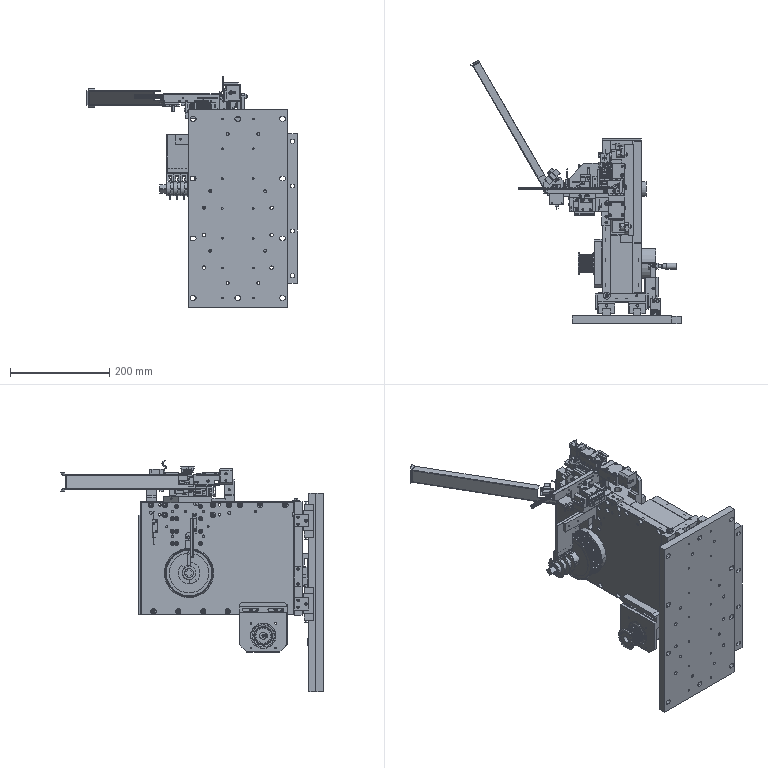Part | NX | 197 solids | 17824 faces | volume 6383940 mm3 | plane 8524 | cylinder 6166 | torus 1403 | cone 1287 | sphere 315 | spline 129 | commonest cylinder face diameters 0.2 x628 5 x553 0.8 x359 0.4 x286 0.6 x277 3.3 x266